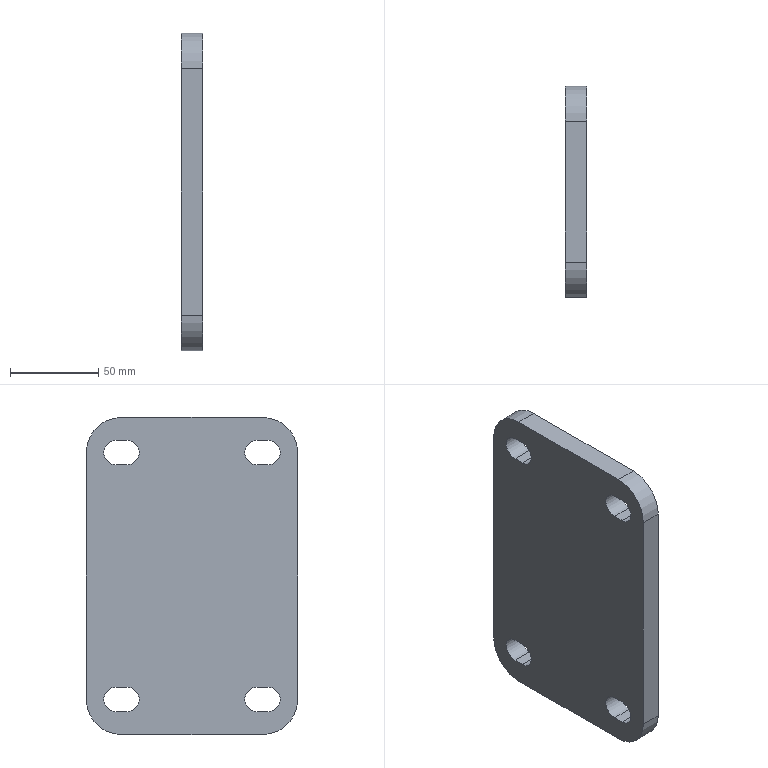Part | STEP file | fixing plate--000.001--20240925 | 1 solid | 26 faces | box 12 x 120 x 180 mm | volume 243659 mm3 | plane 14 | cylinder 12 | commonest cylinder face diameters 14 x8 40 x4